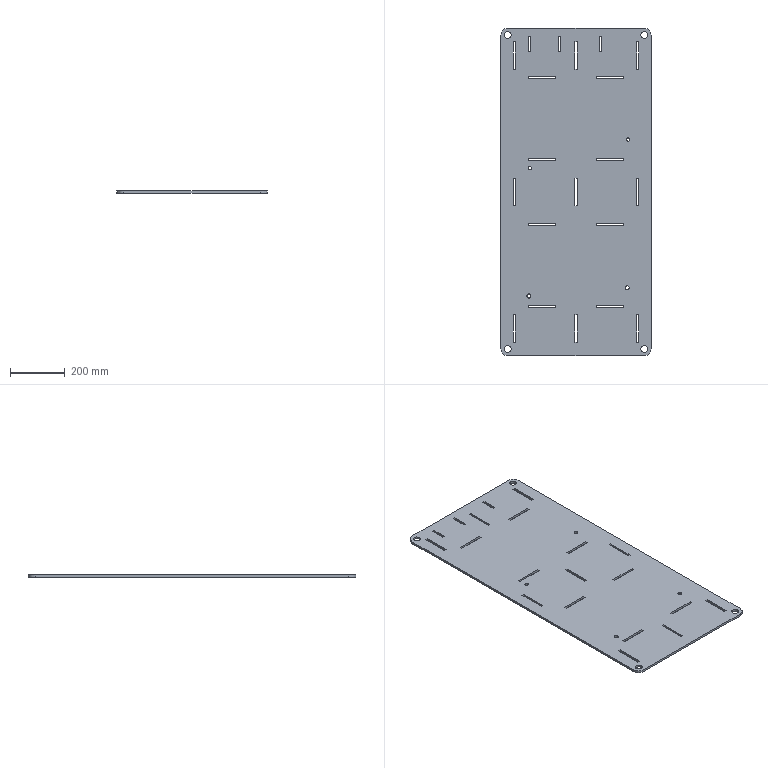Part | SolidWorks | features FlatPattern 1, SMBaseFlange 1, SheetMetal 1 | 1 solid | 106 faces | box 550 x 1200 x 8 mm | volume 5135849 mm3 | plane 86 | cylinder 20 | commonest cylinder face diameters 25 x8 12.5 x4 15 x4 50 x4